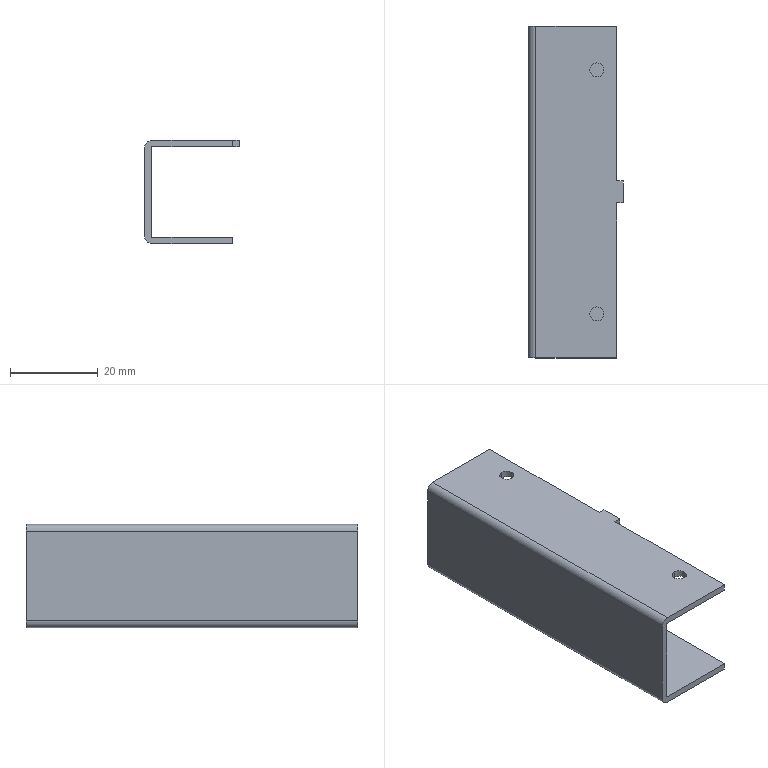Part | STEP file | HESS-408-70-15W-W-25-lower door support bracket 2 | 1 solid | 22 faces | box 21.5 x 75.5 x 23.5 mm | volume 6756 mm3 | plane 14 | cylinder 8 | commonest cylinder face diameters 3.2 x6 0.2 x2